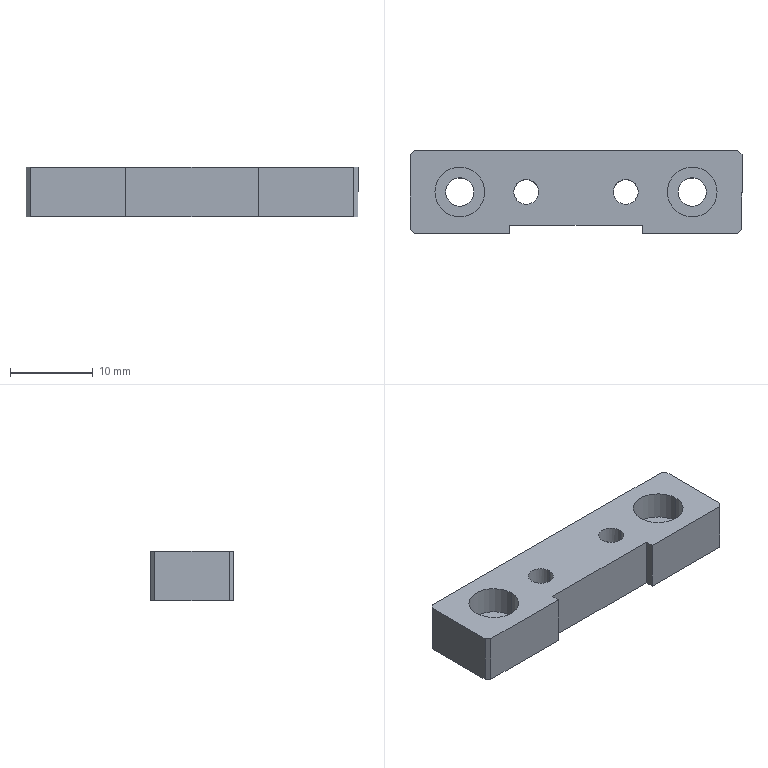Part | SolidWorks | features HoleWzd 2, Chamfer 1, Cut 1, Extrusion 1, ICE 1 | 1 solid | 32 faces | box 40 x 10 x 6 mm | volume 1941 mm3 | cylinder 16 | plane 16 | commonest cylinder face diameters 2.5 x4 3 x4 3.4 x4 6 x4
STEP:
#1=CARTESIAN_POINT('',(-6.,1.5,4.25));
#2=VERTEX_POINT('',#1);
#3=CARTESIAN_POINT('',(-6.,1.5,1.75));
#4=VERTEX_POINT('',#3);
#5=CARTESIAN_POINT('',(-6.,1.5,4.25));
#6=CARTESIAN_POINT('',(-6.088,1.5,4.25));
#7=CARTESIAN_POINT('',(-6.175,1.492,4.241));
#8=CARTESIAN_POINT('',(-6.343,1.463,4.205));
#9=CARTESIAN_POINT('',(-6.425,1.441,4.178));
#10=CARTESIAN_POINT('',(-6.653,1.36,4.079));
#11=CARTESIAN_POINT('',(-6.785,1.285,3.985));
#12=CARTESIAN_POINT('',(-7.002,1.125,3.764));
#13=CARTESIAN_POINT('',(-7.088,1.037,3.635));
#14=CARTESIAN_POINT('',(-7.181,0.9262,3.417));
#15=CARTESIAN_POINT('',(-7.206,0.8923,3.339));
#16=CARTESIAN_POINT('',(-7.241,0.8437,3.174));
#17=CARTESIAN_POINT('',(-7.25,0.8291,3.086));
#18=CARTESIAN_POINT('',(-7.25,0.8292,2.912));
#19=CARTESIAN_POINT('',(-7.24,0.844,2.824));
#20=CARTESIAN_POINT('',(-7.206,0.8927,2.66));
#21=CARTESIAN_POINT('',(-7.181,0.9265,2.582));
#22=CARTESIAN_POINT('',(-7.087,1.038,2.364));
#23=CARTESIAN_POINT('',(-7.001,1.125,2.235));
#24=CARTESIAN_POINT('',(-6.839,1.245,2.07));
#25=CARTESIAN_POINT('',(-6.779,1.284,2.019));
#26=CARTESIAN_POINT('',(-6.648,1.355,1.928));
#27=CARTESIAN_POINT('',(-6.576,1.387,1.888));
#28=CARTESIAN_POINT('',(-6.424,1.441,1.821));
#29=CARTESIAN_POINT('',(-6.342,1.463,1.795));
#30=CARTESIAN_POINT('',(-6.174,1.492,1.759));
#31=CARTESIAN_POINT('',(-6.088,1.5,1.75));
#32=CARTESIAN_POINT('',(-6.,1.5,1.75));
#33=B_SPLINE_CURVE_WITH_KNOTS('',3,(#5,#6,#7,#8,#9,#10,#11,#12,#13,#14,#15,#16,#17,#18,#19,#20,#21,#22,#23,#24,#25,#26,#27,#28,#29,#30,#31,#32),.UNSPECIFIED.,.F.,.F.,(4,2,2,2,2,2,2,2,2,2,2,2,2,4),(0.,0.0002609,0.0005218,0.001044,0.001565,0.001826,0.002087,0.002348,0.002609,0.003131,0.003391,0.003652,0.003913,0.004174),.UNSPECIFIED.);
#34=EDGE_CURVE('',#2,#4,#33,.T.);
#35=ORIENTED_EDGE('',*,*,#34,.T.);
#36=CARTESIAN_POINT('',(-6.,5.,1.75));
#37=VERTEX_POINT('',#36);
#38=CARTESIAN_POINT('',(-6.,5.,1.75));
#39=DIRECTION('',(0.,1.,0.));
#40=VECTOR('',#39,1000.);
#41=LINE('',#38,#40);
#42=EDGE_CURVE('',#4,#37,#41,.T.);
#43=ORIENTED_EDGE('',*,*,#42,.T.);
#44=CARTESIAN_POINT('',(-6.,5.,4.25));
#45=VERTEX_POINT('',#44);
#46=CARTESIAN_POINT('',(-6.,5.,3.));
#47=DIRECTION('',(0.,1.,0.));
#48=DIRECTION('',(0.,0.,1.));
#49=AXIS2_PLACEMENT_3D('',#46,#47,#48);
#50=CIRCLE('',#49,1.25);
#51=EDGE_CURVE('',#37,#45,#50,.T.);
#52=ORIENTED_EDGE('',*,*,#51,.T.);
#53=CARTESIAN_POINT('',(-6.,5.,4.25));
#54=DIRECTION('',(0.,1.,0.));
#55=VECTOR('',#54,1000.);
#56=LINE('',#53,#55);
#57=EDGE_CURVE('',#2,#45,#56,.T.);
#58=ORIENTED_EDGE('',*,*,#57,.F.);
#59=EDGE_LOOP('',(#35,#43,#52,#58));
#60=FACE_OUTER_BOUND('',#59,.T.);
#61=CARTESIAN_POINT('',(-6.,5.,3.));
#62=DIRECTION('',(0.,1.,0.));
#63=DIRECTION('',(0.,0.,1.));
#64=AXIS2_PLACEMENT_3D('',#61,#62,#63);
#65=CYLINDRICAL_SURFACE('',#64,1.25);
#66=ADVANCED_FACE('',(#60),#65,.F.);
#67=CARTESIAN_POINT('',(6.,1.5,4.25));
#68=VERTEX_POINT('',#67);
#69=CARTESIAN_POINT('',(6.,1.5,1.75));
#70=VERTEX_POINT('',#69);
#71=CARTESIAN_POINT('',(6.,1.5,4.25));
#72=CARTESIAN_POINT('',(5.912,1.5,4.25));
#73=CARTESIAN_POINT('',(5.825,1.492,4.241));
#74=CARTESIAN_POINT('',(5.657,1.463,4.205));
#75=CARTESIAN_POINT('',(5.575,1.441,4.178));
#76=CARTESIAN_POINT('',(5.347,1.36,4.079));
#77=CARTESIAN_POINT('',(5.215,1.285,3.985));
#78=CARTESIAN_POINT('',(4.998,1.125,3.764));
#79=CARTESIAN_POINT('',(4.912,1.037,3.635));
#80=CARTESIAN_POINT('',(4.819,0.9262,3.417));
#81=CARTESIAN_POINT('',(4.794,0.8923,3.339));
#82=CARTESIAN_POINT('',(4.759,0.8437,3.174));
#83=CARTESIAN_POINT('',(4.75,0.8291,3.086));
#84=CARTESIAN_POINT('',(4.75,0.8292,2.912));
#85=CARTESIAN_POINT('',(4.76,0.844,2.824));
#86=CARTESIAN_POINT('',(4.794,0.8927,2.66));
#87=CARTESIAN_POINT('',(4.819,0.9265,2.582));
#88=CARTESIAN_POINT('',(4.913,1.038,2.364));
#89=CARTESIAN_POINT('',(4.999,1.125,2.235));
#90=CARTESIAN_POINT('',(5.161,1.245,2.07));
#91=CARTESIAN_POINT('',(5.221,1.284,2.019));
#92=CARTESIAN_POINT('',(5.352,1.355,1.928));
#93=CARTESIAN_POINT('',(5.424,1.387,1.888));
#94=CARTESIAN_POINT('',(5.576,1.441,1.821));
#95=CARTESIAN_POINT('',(5.658,1.463,1.795));
#96=CARTESIAN_POINT('',(5.826,1.492,1.759));
#97=CARTESIAN_POINT('',(5.912,1.5,1.75));
#98=CARTESIAN_POINT('',(6.,1.5,1.75));
#99=B_SPLINE_CURVE_WITH_KNOTS('',3,(#71,#72,#73,#74,#75,#76,#77,#78,#79,#80,#81,#82,#83,#84,#85,#86,#87,#88,#89,#90,#91,#92,#93,#94,#95,#96,#97,#98),.UNSPECIFIED.,.F.,.F.,(4,2,2,2,2,2,2,2,2,2,2,2,2,4),(0.,0.0002609,0.0005218,0.001044,0.001565,0.001826,0.002087,0.002348,0.002609,0.003131,0.003391,0.003652,0.003913,0.004174),.UNSPECIFIED.);
#100=EDGE_CURVE('',#68,#70,#99,.T.);
#101=ORIENTED_EDGE('',*,*,#100,.T.);
#102=CARTESIAN_POINT('',(6.,5.,1.75));
#103=VERTEX_POINT('',#102);
#104=CARTESIAN_POINT('',(6.,5.,1.75));
#105=DIRECTION('',(0.,1.,0.));
#106=VECTOR('',#105,1000.);
#107=LINE('',#104,#106);
#108=EDGE_CURVE('',#70,#103,#107,.T.);
#109=ORIENTED_EDGE('',*,*,#108,.T.);
#110=CARTESIAN_POINT('',(6.,5.,4.25));
#111=VERTEX_POINT('',#110);
#112=CARTESIAN_POINT('',(6.,5.,3.));
#113=DIRECTION('',(0.,1.,0.));
#114=DIRECTION('',(0.,0.,1.));
#115=AXIS2_PLACEMENT_3D('',#112,#113,#114);
#116=CIRCLE('',#115,1.25);
#117=EDGE_CURVE('',#103,#111,#116,.T.);
#118=ORIENTED_EDGE('',*,*,#117,.T.);
#119=CARTESIAN_POINT('',(6.,5.,4.25));
#120=DIRECTION('',(0.,1.,0.));
#121=VECTOR('',#120,1000.);
#122=LINE('',#119,#121);
#123=EDGE_CURVE('',#68,#111,#122,.T.);
#124=ORIENTED_EDGE('',*,*,#123,.F.);
#125=EDGE_LOOP('',(#101,#109,#118,#124));
#126=FACE_OUTER_BOUND('',#125,.T.);
#127=CARTESIAN_POINT('',(6.,5.,3.));
#128=DIRECTION('',(0.,1.,0.));
#129=DIRECTION('',(0.,0.,1.));
#130=AXIS2_PLACEMENT_3D('',#127,#128,#129);
#131=CYLINDRICAL_SURFACE('',#130,1.25);
#132=ADVANCED_FACE('',(#126),#131,.F.);
#133=CARTESIAN_POINT('',(4.5,0.,6.));
#134=VERTEX_POINT('',#133);
#135=CARTESIAN_POINT('',(7.5,0.,6.));
#136=VERTEX_POINT('',#135);
#137=CARTESIAN_POINT('',(6.,0.,6.));
#138=DIRECTION('',(0.,0.,1.));
#139=DIRECTION('',(1.,0.,0.));
#140=AXIS2_PLACEMENT_3D('',#137,#138,#139);
#141=CIRCLE('',#140,1.5);
#142=EDGE_CURVE('',#134,#136,#141,.T.);
#143=ORIENTED_EDGE('',*,*,#142,.T.);
#144=CARTESIAN_POINT('',(7.5,0.,0.));
#145=VERTEX_POINT('',#144);
#146=CARTESIAN_POINT('',(7.5,0.,6.));
#147=DIRECTION('',(0.,0.,-1.));
#148=VECTOR('',#147,1000.);
#149=LINE('',#146,#148);
#150=EDGE_CURVE('',#136,#145,#149,.T.);
#151=ORIENTED_EDGE('',*,*,#150,.T.);
#152=CARTESIAN_POINT('',(4.5,0.,0.));
#153=VERTEX_POINT('',#152);
#154=CARTESIAN_POINT('',(6.,0.,0.));
#155=DIRECTION('',(0.,0.,1.));
#156=DIRECTION('',(1.,0.,0.));
#157=AXIS2_PLACEMENT_3D('',#154,#155,#156);
#158=CIRCLE('',#157,1.5);
#159=EDGE_CURVE('',#153,#145,#158,.T.);
#160=ORIENTED_EDGE('',*,*,#159,.F.);
#161=CARTESIAN_POINT('',(4.5,0.,6.));
#162=DIRECTION('',(0.,0.,-1.));
#163=VECTOR('',#162,1000.);
#164=LINE('',#161,#163);
#165=EDGE_CURVE('',#134,#153,#164,.T.);
#166=ORIENTED_EDGE('',*,*,#165,.F.);
#167=EDGE_LOOP('',(#143,#151,#160,#166));
#168=FACE_OUTER_BOUND('',#167,.T.);
#169=CARTESIAN_POINT('',(6.,0.,6.));
#170=DIRECTION('',(0.,0.,-1.));
#171=DIRECTION('',(-1.,0.,0.));
#172=AXIS2_PLACEMENT_3D('',#169,#170,#171);
#173=CYLINDRICAL_SURFACE('',#172,1.5);
#174=ADVANCED_FACE('',(#168),#173,.F.);
#175=CARTESIAN_POINT('',(-7.5,0.,6.));
#176=VERTEX_POINT('',#175);
#177=CARTESIAN_POINT('',(-4.5,0.,6.));
#178=VERTEX_POINT('',#177);
#179=CARTESIAN_POINT('',(-6.,0.,6.));
#180=DIRECTION('',(0.,0.,1.));
#181=DIRECTION('',(1.,0.,0.));
#182=AXIS2_PLACEMENT_3D('',#179,#180,#181);
#183=CIRCLE('',#182,1.5);
#184=EDGE_CURVE('',#176,#178,#183,.T.);
#185=ORIENTED_EDGE('',*,*,#184,.T.);
#186=CARTESIAN_POINT('',(-4.5,0.,0.));
#187=VERTEX_POINT('',#186);
#188=CARTESIAN_POINT('',(-4.5,0.,6.));
#189=DIRECTION('',(0.,0.,-1.));
#190=VECTOR('',#189,1000.);
#191=LINE('',#188,#190);
#192=EDGE_CURVE('',#178,#187,#191,.T.);
#193=ORIENTED_EDGE('',*,*,#192,.T.);
#194=CARTESIAN_POINT('',(-7.5,0.,0.));
#195=VERTEX_POINT('',#194);
#196=CARTESIAN_POINT('',(-6.,0.,0.));
#197=DIRECTION('',(0.,0.,1.));
#198=DIRECTION('',(1.,0.,0.));
#199=AXIS2_PLACEMENT_3D('',#196,#197,#198);
#200=CIRCLE('',#199,1.5);
#201=EDGE_CURVE('',#195,#187,#200,.T.);
#202=ORIENTED_EDGE('',*,*,#201,.F.);
#203=CARTESIAN_POINT('',(-7.5,0.,6.));
#204=DIRECTION('',(0.,0.,-1.));
#205=VECTOR('',#204,1000.);
#206=LINE('',#203,#205);
#207=EDGE_CURVE('',#176,#195,#206,.T.);
#208=ORIENTED_EDGE('',*,*,#207,.F.);
#209=EDGE_LOOP('',(#185,#193,#202,#208));
#210=FACE_OUTER_BOUND('',#209,.T.);
#211=CARTESIAN_POINT('',(-6.,0.,6.));
#212=DIRECTION('',(0.,0.,-1.));
#213=DIRECTION('',(-1.,0.,0.));
#214=AXIS2_PLACEMENT_3D('',#211,#212,#213);
#215=CYLINDRICAL_SURFACE('',#214,1.5);
#216=ADVANCED_FACE('',(#210),#215,.F.);
#217=CARTESIAN_POINT('',(-17.,0.,2.6));
#218=VERTEX_POINT('',#217);
#219=CARTESIAN_POINT('',(-11.,0.,2.6));
#220=VERTEX_POINT('',#219);
#221=CARTESIAN_POINT('',(-14.,0.,2.6));
#222=DIRECTION('',(0.,0.,1.));
#223=DIRECTION('',(1.,0.,0.));
#224=AXIS2_PLACEMENT_3D('',#221,#222,#223);
#225=CIRCLE('',#224,3.);
#226=EDGE_CURVE('',#218,#220,#225,.T.);
#227=ORIENTED_EDGE('',*,*,#226,.F.);
#228=CARTESIAN_POINT('',(-17.,0.,6.));
#229=VERTEX_POINT('',#228);
#230=CARTESIAN_POINT('',(-17.,0.,6.));
#231=DIRECTION('',(0.,0.,1.));
#232=VECTOR('',#231,1000.);
#233=LINE('',#230,#232);
#234=EDGE_CURVE('',#218,#229,#233,.T.);
#235=ORIENTED_EDGE('',*,*,#234,.T.);
#236=CARTESIAN_POINT('',(-11.,0.,6.));
#237=VERTEX_POINT('',#236);
#238=CARTESIAN_POINT('',(-14.,0.,6.));
#239=DIRECTION('',(0.,0.,1.));
#240=DIRECTION('',(1.,0.,0.));
#241=AXIS2_PLACEMENT_3D('',#238,#239,#240);
#242=CIRCLE('',#241,3.);
#243=EDGE_CURVE('',#229,#237,#242,.T.);
#244=ORIENTED_EDGE('',*,*,#243,.T.);
#245=CARTESIAN_POINT('',(-11.,0.,6.));
#246=DIRECTION('',(0.,0.,1.));
#247=VECTOR('',#246,1000.);
#248=LINE('',#245,#247);
#249=EDGE_CURVE('',#220,#237,#248,.T.);
#250=ORIENTED_EDGE('',*,*,#249,.F.);
#251=EDGE_LOOP('',(#227,#235,#244,#250));
#252=FACE_OUTER_BOUND('',#251,.T.);
#253=CARTESIAN_POINT('',(-14.,0.,6.));
#254=DIRECTION('',(0.,0.,1.));
#255=DIRECTION('',(1.,0.,0.));
#256=AXIS2_PLACEMENT_3D('',#253,#254,#255);
#257=CYLINDRICAL_SURFACE('',#256,3.);
#258=ADVANCED_FACE('',(#252),#257,.F.);
#259=CARTESIAN_POINT('',(-15.7,0.,0.));
#260=VERTEX_POINT('',#259);
#261=CARTESIAN_POINT('',(-12.3,0.,0.));
#262=VERTEX_POINT('',#261);
#263=CARTESIAN_POINT('',(-14.,0.,0.));
#264=DIRECTION('',(0.,0.,1.));
#265=DIRECTION('',(1.,0.,0.));
#266=AXIS2_PLACEMENT_3D('',#263,#264,#265);
#267=CIRCLE('',#266,1.7);
#268=EDGE_CURVE('',#260,#262,#267,.T.);
#269=ORIENTED_EDGE('',*,*,#268,.F.);
#270=CARTESIAN_POINT('',(-15.7,0.,2.6));
#271=VERTEX_POINT('',#270);
#272=CARTESIAN_POINT('',(-15.7,0.,6.));
#273=DIRECTION('',(0.,0.,1.));
#274=VECTOR('',#273,1000.);
#275=LINE('',#272,#274);
#276=EDGE_CURVE('',#260,#271,#275,.T.);
#277=ORIENTED_EDGE('',*,*,#276,.T.);
#278=CARTESIAN_POINT('',(-12.3,0.,2.6));
#279=VERTEX_POINT('',#278);
#280=CARTESIAN_POINT('',(-14.,0.,2.6));
#281=DIRECTION('',(0.,0.,1.));
#282=DIRECTION('',(1.,0.,0.));
#283=AXIS2_PLACEMENT_3D('',#280,#281,#282);
#284=CIRCLE('',#283,1.7);
#285=EDGE_CURVE('',#271,#279,#284,.T.);
#286=ORIENTED_EDGE('',*,*,#285,.T.);
#287=CARTESIAN_POINT('',(-12.3,0.,6.));
#288=DIRECTION('',(0.,0.,1.));
#289=VECTOR('',#288,1000.);
#290=LINE('',#287,#289);
#291=EDGE_CURVE('',#262,#279,#290,.T.);
#292=ORIENTED_EDGE('',*,*,#291,.F.);
#293=EDGE_LOOP('',(#269,#277,#286,#292));
#294=FACE_OUTER_BOUND('',#293,.T.);
#295=CARTESIAN_POINT('',(-14.,0.,6.));
#296=DIRECTION('',(0.,0.,1.));
#297=DIRECTION('',(1.,0.,0.));
#298=AXIS2_PLACEMENT_3D('',#295,#296,#297);
#299=CYLINDRICAL_SURFACE('',#298,1.7);
#300=ADVANCED_FACE('',(#294),#299,.F.);
#301=CARTESIAN_POINT('',(11.,0.,2.6));
#302=VERTEX_POINT('',#301);
#303=CARTESIAN_POINT('',(17.,0.,2.6));
#304=VERTEX_POINT('',#303);
#305=CARTESIAN_POINT('',(14.,0.,2.6));
#306=DIRECTION('',(0.,0.,1.));
#307=DIRECTION('',(1.,0.,0.));
#308=AXIS2_PLACEMENT_3D('',#305,#306,#307);
#309=CIRCLE('',#308,3.);
#310=EDGE_CURVE('',#302,#304,#309,.T.);
#311=ORIENTED_EDGE('',*,*,#310,.F.);
#312=CARTESIAN_POINT('',(11.,0.,6.));
#313=VERTEX_POINT('',#312);
#314=CARTESIAN_POINT('',(11.,0.,6.));
#315=DIRECTION('',(0.,0.,1.));
#316=VECTOR('',#315,1000.);
#317=LINE('',#314,#316);
#318=EDGE_CURVE('',#302,#313,#317,.T.);
#319=ORIENTED_EDGE('',*,*,#318,.T.);
#320=CARTESIAN_POINT('',(17.,0.,6.));
#321=VERTEX_POINT('',#320);
#322=CARTESIAN_POINT('',(14.,0.,6.));
#323=DIRECTION('',(0.,0.,1.));
#324=DIRECTION('',(1.,0.,0.));
#325=AXIS2_PLACEMENT_3D('',#322,#323,#324);
#326=CIRCLE('',#325,3.);
#327=EDGE_CURVE('',#313,#321,#326,.T.);
#328=ORIENTED_EDGE('',*,*,#327,.T.);
#329=CARTESIAN_POINT('',(17.,0.,6.));
#330=DIRECTION('',(0.,0.,1.));
#331=VECTOR('',#330,1000.);
#332=LINE('',#329,#331);
#333=EDGE_CURVE('',#304,#321,#332,.T.);
#334=ORIENTED_EDGE('',*,*,#333,.F.);
#335=EDGE_LOOP('',(#311,#319,#328,#334));
#336=FACE_OUTER_BOUND('',#335,.T.);
#337=CARTESIAN_POINT('',(14.,0.,6.));
#338=DIRECTION('',(0.,0.,1.));
#339=DIRECTION('',(1.,0.,0.));
#340=AXIS2_PLACEMENT_3D('',#337,#338,#339);
#341=CYLINDRICAL_SURFACE('',#340,3.);
#342=ADVANCED_FACE('',(#336),#341,.F.);
#343=CARTESIAN_POINT('',(12.3,0.,0.));
#344=VERTEX_POINT('',#343);
#345=CARTESIAN_POINT('',(15.7,0.,0.));
#346=VERTEX_POINT('',#345);
#347=CARTESIAN_POINT('',(14.,0.,0.));
#348=DIRECTION('',(0.,0.,1.));
#349=DIRECTION('',(1.,0.,0.));
#350=AXIS2_PLACEMENT_3D('',#347,#348,#349);
#351=CIRCLE('',#350,1.7);
#352=EDGE_CURVE('',#344,#346,#351,.T.);
#353=ORIENTED_EDGE('',*,*,#352,.F.);
#354=CARTESIAN_POINT('',(12.3,0.,2.6));
#355=VERTEX_POINT('',#354);
#356=CARTESIAN_POINT('',(12.3,0.,6.));
#357=DIRECTION('',(0.,0.,1.));
#358=VECTOR('',#357,1000.);
#359=LINE('',#356,#358);
#360=EDGE_CURVE('',#344,#355,#359,.T.);
#361=ORIENTED_EDGE('',*,*,#360,.T.);
#362=CARTESIAN_POINT('',(15.7,0.,2.6));
#363=VERTEX_POINT('',#362);
#364=CARTESIAN_POINT('',(14.,0.,2.6));
#365=DIRECTION('',(0.,0.,1.));
#366=DIRECTION('',(1.,0.,0.));
#367=AXIS2_PLACEMENT_3D('',#364,#365,#366);
#368=CIRCLE('',#367,1.7);
#369=EDGE_CURVE('',#355,#363,#368,.T.);
#370=ORIENTED_EDGE('',*,*,#369,.T.);
#371=CARTESIAN_POINT('',(15.7,0.,6.));
#372=DIRECTION('',(0.,0.,1.));
#373=VECTOR('',#372,1000.);
#374=LINE('',#371,#373);
#375=EDGE_CURVE('',#346,#363,#374,.T.);
#376=ORIENTED_EDGE('',*,*,#375,.F.);
#377=EDGE_LOOP('',(#353,#361,#370,#376));
#378=FACE_OUTER_BOUND('',#377,.T.);
#379=CARTESIAN_POINT('',(14.,0.,6.));
#380=DIRECTION('',(0.,0.,1.));
#381=DIRECTION('',(1.,0.,0.));
#382=AXIS2_PLACEMENT_3D('',#379,#380,#381);
#383=CYLINDRICAL_SURFACE('',#382,1.7);
#384=ADVANCED_FACE('',(#378),#383,.F.);
#385=ORIENTED_EDGE('',*,*,#184,.F.);
#386=CARTESIAN_POINT('',(-6.,0.,6.));
#387=DIRECTION('',(0.,0.,1.));
#388=DIRECTION('',(1.,0.,0.));
#389=AXIS2_PLACEMENT_3D('',#386,#387,#388);
#390=CIRCLE('',#389,1.5);
#391=EDGE_CURVE('',#178,#176,#390,.T.);
#392=ORIENTED_EDGE('',*,*,#391,.F.);
#393=EDGE_LOOP('',(#385,#392));
#394=FACE_BOUND('',#393,.T.);
#395=CARTESIAN_POINT('',(14.,0.,6.));
#396=DIRECTION('',(0.,0.,1.));
#397=DIRECTION('',(1.,0.,0.));
#398=AXIS2_PLACEMENT_3D('',#395,#396,#397);
#399=CIRCLE('',#398,3.);
#400=EDGE_CURVE('',#321,#313,#399,.T.);
#401=ORIENTED_EDGE('',*,*,#400,.F.);
#402=ORIENTED_EDGE('',*,*,#327,.F.);
#403=EDGE_LOOP('',(#401,#402));
#404=FACE_BOUND('',#403,.T.);
#405=CARTESIAN_POINT('',(-14.,0.,6.));
#406=DIRECTION('',(0.,0.,1.));
#407=DIRECTION('',(1.,0.,0.));
#408=AXIS2_PLACEMENT_3D('',#405,#406,#407);
#409=CIRCLE('',#408,3.);
#410=EDGE_CURVE('',#237,#229,#409,.T.);
#411=ORIENTED_EDGE('',*,*,#410,.F.);
#412=ORIENTED_EDGE('',*,*,#243,.F.);
#413=EDGE_LOOP('',(#411,#412));
#414=FACE_BOUND('',#413,.T.);
#415=CARTESIAN_POINT('',(-19.5,-5.,6.));
#416=VERTEX_POINT('',#415);
#417=CARTESIAN_POINT('',(-8.,-5.,6.));
#418=VERTEX_POINT('',#417);
#419=CARTESIAN_POINT('',(20.,-5.,6.));
#420=DIRECTION('',(1.,0.,0.));
#421=VECTOR('',#420,1000.);
#422=LINE('',#419,#421);
#423=EDGE_CURVE('',#416,#418,#422,.T.);
#424=ORIENTED_EDGE('',*,*,#423,.T.);
#425=CARTESIAN_POINT('',(-8.,-4.,6.));
#426=VERTEX_POINT('',#425);
#427=CARTESIAN_POINT('',(-8.,-4.,6.));
#428=DIRECTION('',(0.,-1.,0.));
#429=VECTOR('',#428,1000.);
#430=LINE('',#427,#429);
#431=EDGE_CURVE('',#426,#418,#430,.T.);
#432=ORIENTED_EDGE('',*,*,#431,.F.);
#433=CARTESIAN_POINT('',(8.,-4.,6.));
#434=VERTEX_POINT('',#433);
#435=CARTESIAN_POINT('',(8.,-4.,6.));
#436=DIRECTION('',(1.,0.,0.));
#437=VECTOR('',#436,1000.);
#438=LINE('',#435,#437);
#439=EDGE_CURVE('',#426,#434,#438,.T.);
#440=ORIENTED_EDGE('',*,*,#439,.T.);
#441=CARTESIAN_POINT('',(8.,-5.,6.));
#442=VERTEX_POINT('',#441);
#443=CARTESIAN_POINT('',(8.,-4.,6.));
#444=DIRECTION('',(0.,-1.,0.));
#445=VECTOR('',#444,1000.);
#446=LINE('',#443,#445);
#447=EDGE_CURVE('',#434,#442,#446,.T.);
#448=ORIENTED_EDGE('',*,*,#447,.T.);
#449=CARTESIAN_POINT('',(19.5,-5.,6.));
#450=VERTEX_POINT('',#449);
#451=CARTESIAN_POINT('',(20.,-5.,6.));
#452=DIRECTION('',(1.,0.,0.));
#453=VECTOR('',#452,1000.);
#454=LINE('',#451,#453);
#455=EDGE_CURVE('',#442,#450,#454,.T.);
#456=ORIENTED_EDGE('',*,*,#455,.T.);
#457=CARTESIAN_POINT('',(20.,-4.5,6.));
#458=VERTEX_POINT('',#457);
#459=CARTESIAN_POINT('',(4.75,-19.75,6.));
#460=DIRECTION('',(0.7071,0.7071,0.));
#461=VECTOR('',#460,1000.);
#462=LINE('',#459,#461);
#463=EDGE_CURVE('',#450,#458,#462,.T.);
#464=ORIENTED_EDGE('',*,*,#463,.T.);
#465=CARTESIAN_POINT('',(20.,4.5,6.));
#466=VERTEX_POINT('',#465);
#467=CARTESIAN_POINT('',(20.,-5.,6.));
#468=DIRECTION('',(0.,1.,0.));
#469=VECTOR('',#468,1000.);
#470=LINE('',#467,#469);
#471=EDGE_CURVE('',#458,#466,#470,.T.);
#472=ORIENTED_EDGE('',*,*,#471,.T.);
#473=CARTESIAN_POINT('',(19.5,5.,6.));
#474=VERTEX_POINT('',#473);
#475=CARTESIAN_POINT('',(-0.25,24.75,6.));
#476=DIRECTION('',(-0.7071,0.7071,0.));
#477=VECTOR('',#476,1000.);
#478=LINE('',#475,#477);
#479=EDGE_CURVE('',#466,#474,#478,.T.);
#480=ORIENTED_EDGE('',*,*,#479,.T.);
#481=CARTESIAN_POINT('',(-19.5,5.,6.));
#482=VERTEX_POINT('',#481);
#483=CARTESIAN_POINT('',(20.,5.,6.));
#484=DIRECTION('',(-1.,0.,0.));
#485=VECTOR('',#484,1000.);
#486=LINE('',#483,#485);
#487=EDGE_CURVE('',#474,#482,#486,.T.);
#488=ORIENTED_EDGE('',*,*,#487,.T.);
#489=CARTESIAN_POINT('',(-20.,4.5,6.));
#490=VERTEX_POINT('',#489);
#491=CARTESIAN_POINT('',(-19.75,4.75,6.));
#492=DIRECTION('',(-0.7071,-0.7071,0.));
#493=VECTOR('',#492,1000.);
#494=LINE('',#491,#493);
#495=EDGE_CURVE('',#482,#490,#494,.T.);
#496=ORIENTED_EDGE('',*,*,#495,.T.);
#497=CARTESIAN_POINT('',(-20.,-4.5,6.));
#498=VERTEX_POINT('',#497);
#499=CARTESIAN_POINT('',(-20.,-5.,6.));
#500=DIRECTION('',(0.,-1.,0.));
#501=VECTOR('',#500,1000.);
#502=LINE('',#499,#501);
#503=EDGE_CURVE('',#490,#498,#502,.T.);
#504=ORIENTED_EDGE('',*,*,#503,.T.);
#505=CARTESIAN_POINT('',(-24.75,0.25,6.));
#506=DIRECTION('',(0.7071,-0.7071,0.));
#507=VECTOR('',#506,1000.);
#508=LINE('',#505,#507);
#509=EDGE_CURVE('',#498,#416,#508,.T.);
#510=ORIENTED_EDGE('',*,*,#509,.T.);
#511=EDGE_LOOP('',(#424,#432,#440,#448,#456,#464,#472,#480,#488,#496,#504,#510));
#512=FACE_OUTER_BOUND('',#511,.T.);
#513=ORIENTED_EDGE('',*,*,#142,.F.);
#514=CARTESIAN_POINT('',(6.,0.,6.));
#515=DIRECTION('',(0.,0.,1.));
#516=DIRECTION('',(1.,0.,0.));
#517=AXIS2_PLACEMENT_3D('',#514,#515,#516);
#518=CIRCLE('',#517,1.5);
#519=EDGE_CURVE('',#136,#134,#518,.T.);
#520=ORIENTED_EDGE('',*,*,#519,.F.);
#521=EDGE_LOOP('',(#513,#520));
#522=FACE_BOUND('',#521,.T.);
#523=CARTESIAN_POINT('',(-20.,5.,6.));
#524=DIRECTION('',(0.,0.,1.));
#525=DIRECTION('',(1.,0.,0.));
#526=AXIS2_PLACEMENT_3D('',#523,#524,#525);
#527=PLANE('',#526);
#528=ADVANCED_FACE('',(#394,#404,#414,#512,#522),#527,.T.);
#529=ORIENTED_EDGE('',*,*,#201,.T.);
#530=CARTESIAN_POINT('',(-6.,0.,0.));
#531=DIRECTION('',(0.,0.,1.));
#532=DIRECTION('',(1.,0.,0.));
#533=AXIS2_PLACEMENT_3D('',#530,#531,#532);
#534=CIRCLE('',#533,1.5);
#535=EDGE_CURVE('',#187,#195,#534,.T.);
#536=ORIENTED_EDGE('',*,*,#535,.T.);
#537=EDGE_LOOP('',(#529,#536));
#538=FACE_BOUND('',#537,.T.);
#539=CARTESIAN_POINT('',(14.,0.,0.));
#540=DIRECTION('',(0.,0.,1.));
#541=DIRECTION('',(1.,0.,0.));
#542=AXIS2_PLACEMENT_3D('',#539,#540,#541);
#543=CIRCLE('',#542,1.7);
#544=EDGE_CURVE('',#346,#344,#543,.T.);
#545=ORIENTED_EDGE('',*,*,#544,.T.);
#546=ORIENTED_EDGE('',*,*,#352,.T.);
#547=EDGE_LOOP('',(#545,#546));
#548=FACE_BOUND('',#547,.T.);
#549=CARTESIAN_POINT('',(-14.,0.,0.));
#550=DIRECTION('',(0.,0.,1.));
#551=DIRECTION('',(1.,0.,0.));
#552=AXIS2_PLACEMENT_3D('',#549,#550,#551);
#553=CIRCLE('',#552,1.7);
#554=EDGE_CURVE('',#262,#260,#553,.T.);
#555=ORIENTED_EDGE('',*,*,#554,.T.);
#556=ORIENTED_EDGE('',*,*,#268,.T.);
#557=EDGE_LOOP('',(#555,#556));
#558=FACE_BOUND('',#557,.T.);
#559=CARTESIAN_POINT('',(-8.,-4.,0.));
#560=VERTEX_POINT('',#559);
#561=CARTESIAN_POINT('',(-8.,-5.,0.));
#562=VERTEX_POINT('',#561);
#563=CARTESIAN_POINT('',(-8.,-4.,0.));
#564=DIRECTION('',(0.,-1.,0.));
#565=VECTOR('',#564,1000.);
#566=LINE('',#563,#565);
#567=EDGE_CURVE('',#560,#562,#566,.T.);
#568=ORIENTED_EDGE('',*,*,#567,.T.);
#569=CARTESIAN_POINT('',(-19.5,-5.,0.));
#570=VERTEX_POINT('',#569);
#571=CARTESIAN_POINT('',(20.,-5.,0.));
#572=DIRECTION('',(1.,0.,0.));
#573=VECTOR('',#572,1000.);
#574=LINE('',#571,#573);
#575=EDGE_CURVE('',#570,#562,#574,.T.);
#576=ORIENTED_EDGE('',*,*,#575,.F.);
#577=CARTESIAN_POINT('',(-20.,-4.5,0.));
#578=VERTEX_POINT('',#577);
#579=CARTESIAN_POINT('',(-19.5,-5.,0.));
#580=DIRECTION('',(-0.7071,0.7071,0.));
#581=VECTOR('',#580,1000.);
#582=LINE('',#579,#581);
#583=EDGE_CURVE('',#570,#578,#582,.T.);
#584=ORIENTED_EDGE('',*,*,#583,.T.);
#585=CARTESIAN_POINT('',(-20.,4.5,0.));
#586=VERTEX_POINT('',#585);
#587=CARTESIAN_POINT('',(-20.,-5.,0.));
#588=DIRECTION('',(0.,-1.,0.));
#589=VECTOR('',#588,1000.);
#590=LINE('',#587,#589);
#591=EDGE_CURVE('',#586,#578,#590,.T.);
#592=ORIENTED_EDGE('',*,*,#591,.F.);
#593=CARTESIAN_POINT('',(-19.5,5.,0.));
#594=VERTEX_POINT('',#593);
#595=CARTESIAN_POINT('',(-20.,4.5,0.));
#596=DIRECTION('',(0.7071,0.7071,0.));
#597=VECTOR('',#596,1000.);
#598=LINE('',#595,#597);
#599=EDGE_CURVE('',#586,#594,#598,.T.);
#600=ORIENTED_EDGE('',*,*,#599,.T.);
#601=CARTESIAN_POINT('',(19.5,5.,0.));
#602=VERTEX_POINT('',#601);
#603=CARTESIAN_POINT('',(20.,5.,0.));
#604=DIRECTION('',(-1.,0.,0.));
#605=VECTOR('',#604,1000.);
#606=LINE('',#603,#605);
#607=EDGE_CURVE('',#602,#594,#606,.T.);
#608=ORIENTED_EDGE('',*,*,#607,.F.);
#609=CARTESIAN_POINT('',(20.,4.5,0.));
#610=VERTEX_POINT('',#609);
#611=CARTESIAN_POINT('',(19.5,5.,0.));
#612=DIRECTION('',(0.7071,-0.7071,0.));
#613=VECTOR('',#612,1000.);
#614=LINE('',#611,#613);
#615=EDGE_CURVE('',#602,#610,#614,.T.);
#616=ORIENTED_EDGE('',*,*,#615,.T.);
#617=CARTESIAN_POINT('',(20.,-4.5,0.));
#618=VERTEX_POINT('',#617);
#619=CARTESIAN_POINT('',(20.,-5.,0.));
#620=DIRECTION('',(0.,1.,0.));
#621=VECTOR('',#620,1000.);
#622=LINE('',#619,#621);
#623=EDGE_CURVE('',#618,#610,#622,.T.);
#624=ORIENTED_EDGE('',*,*,#623,.F.);
#625=CARTESIAN_POINT('',(19.5,-5.,0.));
#626=VERTEX_POINT('',#625);
#627=CARTESIAN_POINT('',(20.,-4.5,0.));
#628=DIRECTION('',(-0.7071,-0.7071,0.));
#629=VECTOR('',#628,1000.);
#630=LINE('',#627,#629);
#631=EDGE_CURVE('',#618,#626,#630,.T.);
#632=ORIENTED_EDGE('',*,*,#631,.T.);
#633=CARTESIAN_POINT('',(8.,-5.,0.));
#634=VERTEX_POINT('',#633);
#635=CARTESIAN_POINT('',(20.,-5.,0.));
#636=DIRECTION('',(1.,0.,0.));
#637=VECTOR('',#636,1000.);
#638=LINE('',#635,#637);
#639=EDGE_CURVE('',#634,#626,#638,.T.);
#640=ORIENTED_EDGE('',*,*,#639,.F.);
#641=CARTESIAN_POINT('',(8.,-4.,0.));
#642=VERTEX_POINT('',#641);
#643=CARTESIAN_POINT('',(8.,-4.,0.));
#644=DIRECTION('',(0.,-1.,0.));
#645=VECTOR('',#644,1000.);
#646=LINE('',#643,#645);
#647=EDGE_CURVE('',#642,#634,#646,.T.);
#648=ORIENTED_EDGE('',*,*,#647,.F.);
#649=CARTESIAN_POINT('',(8.,-4.,0.));
#650=DIRECTION('',(-1.,0.,0.));
#651=VECTOR('',#650,1000.);
#652=LINE('',#649,#651);
#653=EDGE_CURVE('',#642,#560,#652,.T.);
#654=ORIENTED_EDGE('',*,*,#653,.T.);
#655=EDGE_LOOP('',(#568,#576,#584,#592,#600,#608,#616,#624,#632,#640,#648,#654));
#656=FACE_OUTER_BOUND('',#655,.T.);
#657=ORIENTED_EDGE('',*,*,#159,.T.);
#658=CARTESIAN_POINT('',(6.,0.,0.));
#659=DIRECTION('',(0.,0.,1.));
#660=DIRECTION('',(1.,0.,0.));
#661=AXIS2_PLACEMENT_3D('',#658,#659,#660);
#662=CIRCLE('',#661,1.5);
#663=EDGE_CURVE('',#145,#153,#662,.T.);
#664=ORIENTED_EDGE('',*,*,#663,.T.);
#665=EDGE_LOOP('',(#657,#664));
#666=FACE_BOUND('',#665,.T.);
#667=CARTESIAN_POINT('',(-20.,5.,0.));
#668=DIRECTION('',(0.,0.,1.));
#669=DIRECTION('',(1.,0.,0.));
#670=AXIS2_PLACEMENT_3D('',#667,#668,#669);
#671=PLANE('',#670);
#672=ADVANCED_FACE('',(#538,#548,#558,#656,#666),#671,.F.);
#673=CARTESIAN_POINT('',(-8.,-5.,6.));
#674=DIRECTION('',(0.,0.,1.));
#675=VECTOR('',#674,1000.);
#676=LINE('',#673,#675);
#677=EDGE_CURVE('',#562,#418,#676,.T.);
#678=ORIENTED_EDGE('',*,*,#677,.T.);
#679=ORIENTED_EDGE('',*,*,#423,.F.);
#680=CARTESIAN_POINT('',(-19.5,-5.,6.));
#681=DIRECTION('',(0.,0.,-1.));
#682=VECTOR('',#681,1000.);
#683=LINE('',#680,#682);
#684=EDGE_CURVE('',#416,#570,#683,.T.);
#685=ORIENTED_EDGE('',*,*,#684,.T.);
#686=ORIENTED_EDGE('',*,*,#575,.T.);
#687=EDGE_LOOP('',(#678,#679,#685,#686));
#688=FACE_OUTER_BOUND('',#687,.T.);
#689=CARTESIAN_POINT('',(20.,-5.,6.));
#690=DIRECTION('',(0.,1.,0.));
#691=DIRECTION('',(-1.,0.,0.));
#692=AXIS2_PLACEMENT_3D('',#689,#690,#691);
#693=PLANE('',#692);
#694=ADVANCED_FACE('',(#688),#693,.F.);
#695=CARTESIAN_POINT('',(8.,-5.,6.));
#696=DIRECTION('',(0.,0.,-1.));
#697=VECTOR('',#696,1000.);
#698=LINE('',#695,#697);
#699=EDGE_CURVE('',#442,#634,#698,.T.);
#700=ORIENTED_EDGE('',*,*,#699,.T.);
#701=ORIENTED_EDGE('',*,*,#639,.T.);
#702=CARTESIAN_POINT('',(19.5,-5.,6.));
#703=DIRECTION('',(0.,0.,1.));
#704=VECTOR('',#703,1000.);
#705=LINE('',#702,#704);
#706=EDGE_CURVE('',#626,#450,#705,.T.);
#707=ORIENTED_EDGE('',*,*,#706,.T.);
#708=ORIENTED_EDGE('',*,*,#455,.F.);
#709=EDGE_LOOP('',(#700,#701,#707,#708));
#710=FACE_OUTER_BOUND('',#709,.T.);
#711=CARTESIAN_POINT('',(20.,-5.,6.));
#712=DIRECTION('',(0.,1.,0.));
#713=DIRECTION('',(-1.,0.,0.));
#714=AXIS2_PLACEMENT_3D('',#711,#712,#713);
#715=PLANE('',#714);
#716=ADVANCED_FACE('',(#710),#715,.F.);
#717=ORIENTED_EDGE('',*,*,#503,.F.);
#718=CARTESIAN_POINT('',(-20.,4.5,6.));
#719=DIRECTION('',(0.,0.,-1.));
#720=VECTOR('',#719,1000.);
#721=LINE('',#718,#720);
#722=EDGE_CURVE('',#490,#586,#721,.T.);
#723=ORIENTED_EDGE('',*,*,#722,.T.);
#724=ORIENTED_EDGE('',*,*,#591,.T.);
#725=CARTESIAN_POINT('',(-20.,-4.5,6.));
#726=DIRECTION('',(0.,0.,1.));
#727=VECTOR('',#726,1000.);
#728=LINE('',#725,#727);
#729=EDGE_CURVE('',#578,#498,#728,.T.);
#730=ORIENTED_EDGE('',*,*,#729,.T.);
#731=EDGE_LOOP('',(#717,#723,#724,#730));
#732=FACE_OUTER_BOUND('',#731,.T.);
#733=CARTESIAN_POINT('',(-20.,-5.,6.));
#734=DIRECTION('',(1.,0.,0.));
#735=DIRECTION('',(0.,0.,-1.));
#736=AXIS2_PLACEMENT_3D('',#733,#734,#735);
#737=PLANE('',#736);
#738=ADVANCED_FACE('',(#732),#737,.F.);
#739=ORIENTED_EDGE('',*,*,#471,.F.);
#740=CARTESIAN_POINT('',(20.,-4.5,6.));
#741=DIRECTION('',(0.,0.,-1.));
#742=VECTOR('',#741,1000.);
#743=LINE('',#740,#742);
#744=EDGE_CURVE('',#458,#618,#743,.T.);
#745=ORIENTED_EDGE('',*,*,#744,.T.);
#746=ORIENTED_EDGE('',*,*,#623,.T.);
#747=CARTESIAN_POINT('',(20.,4.5,6.));
#748=DIRECTION('',(0.,0.,1.));
#749=VECTOR('',#748,1000.);
#750=LINE('',#747,#749);
#751=EDGE_CURVE('',#610,#466,#750,.T.);
#752=ORIENTED_EDGE('',*,*,#751,.T.);
#753=EDGE_LOOP('',(#739,#745,#746,#752));
#754=FACE_OUTER_BOUND('',#753,.T.);
#755=CARTESIAN_POINT('',(20.,-5.,6.));
#756=DIRECTION('',(-1.,0.,0.));
#757=DIRECTION('',(0.,0.,1.));
#758=AXIS2_PLACEMENT_3D('',#755,#756,#757);
#759=PLANE('',#758);
#760=ADVANCED_FACE('',(#754),#759,.F.);
#761=CARTESIAN_POINT('',(-6.,5.,3.));
#762=DIRECTION('',(0.,1.,0.));
#763=DIRECTION('',(0.,0.,1.));
#764=AXIS2_PLACEMENT_3D('',#761,#762,#763);
#765=CIRCLE('',#764,1.25);
#766=EDGE_CURVE('',#45,#37,#765,.T.);
#767=ORIENTED_EDGE('',*,*,#766,.F.);
#768=ORIENTED_EDGE('',*,*,#51,.F.);
#769=EDGE_LOOP('',(#767,#768));
#770=FACE_BOUND('',#769,.T.);
#771=CARTESIAN_POINT('',(6.,5.,3.));
#772=DIRECTION('',(0.,1.,0.));
#773=DIRECTION('',(0.,0.,1.));
#774=AXIS2_PLACEMENT_3D('',#771,#772,#773);
#775=CIRCLE('',#774,1.25);
#776=EDGE_CURVE('',#111,#103,#775,.T.);
#777=ORIENTED_EDGE('',*,*,#776,.F.);
#778=ORIENTED_EDGE('',*,*,#117,.F.);
#779=EDGE_LOOP('',(#777,#778));
#780=FACE_BOUND('',#779,.T.);
#781=ORIENTED_EDGE('',*,*,#487,.F.);
#782=CARTESIAN_POINT('',(19.5,5.,6.));
#783=DIRECTION('',(0.,0.,-1.));
#784=VECTOR('',#783,1000.);
#785=LINE('',#782,#784);
#786=EDGE_CURVE('',#474,#602,#785,.T.);
#787=ORIENTED_EDGE('',*,*,#786,.T.);
#788=ORIENTED_EDGE('',*,*,#607,.T.);
#789=CARTESIAN_POINT('',(-19.5,5.,6.));
#790=DIRECTION('',(0.,0.,1.));
#791=VECTOR('',#790,1000.);
#792=LINE('',#789,#791);
#793=EDGE_CURVE('',#594,#482,#792,.T.);
#794=ORIENTED_EDGE('',*,*,#793,.T.);
#795=EDGE_LOOP('',(#781,#787,#788,#794));
#796=FACE_OUTER_BOUND('',#795,.T.);
#797=CARTESIAN_POINT('',(20.,5.,6.));
#798=DIRECTION('',(0.,-1.,0.));
#799=DIRECTION('',(1.,0.,0.));
#800=AXIS2_PLACEMENT_3D('',#797,#798,#799);
#801=PLANE('',#800);
#802=ADVANCED_FACE('',(#770,#780,#796),#801,.F.);
#803=ORIENTED_EDGE('',*,*,#463,.F.);
#804=ORIENTED_EDGE('',*,*,#706,.F.);
#805=ORIENTED_EDGE('',*,*,#631,.F.);
#806=ORIENTED_EDGE('',*,*,#744,.F.);
#807=EDGE_LOOP('',(#803,#804,#805,#806));
#808=FACE_OUTER_BOUND('',#807,.T.);
#809=CARTESIAN_POINT('',(20.,-4.5,6.));
#810=DIRECTION('',(-0.7071,0.7071,0.));
#811=DIRECTION('',(-0.7071,-0.7071,0.));
#812=AXIS2_PLACEMENT_3D('',#809,#810,#811);
#813=PLANE('',#812);
#814=ADVANCED_FACE('',(#808),#813,.F.);
#815=ORIENTED_EDGE('',*,*,#479,.F.);
#816=ORIENTED_EDGE('',*,*,#751,.F.);
#817=ORIENTED_EDGE('',*,*,#615,.F.);
#818=ORIENTED_EDGE('',*,*,#786,.F.);
#819=EDGE_LOOP('',(#815,#816,#817,#818));
#820=FACE_OUTER_BOUND('',#819,.T.);
#821=CARTESIAN_POINT('',(19.5,5.,6.));
#822=DIRECTION('',(-0.7071,-0.7071,0.));
#823=DIRECTION('',(0.7071,-0.7071,0.));
#824=AXIS2_PLACEMENT_3D('',#821,#822,#823);
#825=PLANE('',#824);
#826=ADVANCED_FACE('',(#820),#825,.F.);
#827=ORIENTED_EDGE('',*,*,#495,.F.);
#828=ORIENTED_EDGE('',*,*,#793,.F.);
#829=ORIENTED_EDGE('',*,*,#599,.F.);
#830=ORIENTED_EDGE('',*,*,#722,.F.);
#831=EDGE_LOOP('',(#827,#828,#829,#830));
#832=FACE_OUTER_BOUND('',#831,.T.);
#833=CARTESIAN_POINT('',(-20.,4.5,6.));
#834=DIRECTION('',(0.7071,-0.7071,0.));
#835=DIRECTION('',(0.7071,0.7071,0.));
#836=AXIS2_PLACEMENT_3D('',#833,#834,#835);
#837=PLANE('',#836);
#838=ADVANCED_FACE('',(#832),#837,.F.);
#839=ORIENTED_EDGE('',*,*,#509,.F.);
#840=ORIENTED_EDGE('',*,*,#729,.F.);
#841=ORIENTED_EDGE('',*,*,#583,.F.);
#842=ORIENTED_EDGE('',*,*,#684,.F.);
#843=EDGE_LOOP('',(#839,#840,#841,#842));
#844=FACE_OUTER_BOUND('',#843,.T.);
#845=CARTESIAN_POINT('',(-19.5,-5.,6.));
#846=DIRECTION('',(0.7071,0.7071,0.));
#847=DIRECTION('',(-0.7071,0.7071,0.));
#848=AXIS2_PLACEMENT_3D('',#845,#846,#847);
#849=PLANE('',#848);
#850=ADVANCED_FACE('',(#844),#849,.F.);
#851=ORIENTED_EDGE('',*,*,#360,.F.);
#852=ORIENTED_EDGE('',*,*,#544,.F.);
#853=ORIENTED_EDGE('',*,*,#375,.T.);
#854=CARTESIAN_POINT('',(14.,0.,2.6));
#855=DIRECTION('',(0.,0.,1.));
#856=DIRECTION('',(1.,0.,0.));
#857=AXIS2_PLACEMENT_3D('',#854,#855,#856);
#858=CIRCLE('',#857,1.7);
#859=EDGE_CURVE('',#363,#355,#858,.T.);
#860=ORIENTED_EDGE('',*,*,#859,.T.);
#861=EDGE_LOOP('',(#851,#852,#853,#860));
#862=FACE_OUTER_BOUND('',#861,.T.);
#863=CARTESIAN_POINT('',(14.,0.,6.));
#864=DIRECTION('',(0.,0.,1.));
#865=DIRECTION('',(1.,0.,0.));
#866=AXIS2_PLACEMENT_3D('',#863,#864,#865);
#867=CYLINDRICAL_SURFACE('',#866,1.7);
#868=ADVANCED_FACE('',(#862),#867,.F.);
#869=ORIENTED_EDGE('',*,*,#859,.F.);
#870=ORIENTED_EDGE('',*,*,#369,.F.);
#871=EDGE_LOOP('',(#869,#870));
#872=FACE_BOUND('',#871,.T.);
#873=CARTESIAN_POINT('',(14.,0.,2.6));
#874=DIRECTION('',(0.,0.,1.));
#875=DIRECTION('',(1.,0.,0.));
#876=AXIS2_PLACEMENT_3D('',#873,#874,#875);
#877=CIRCLE('',#876,3.);
#878=EDGE_CURVE('',#304,#302,#877,.T.);
#879=ORIENTED_EDGE('',*,*,#878,.T.);
#880=ORIENTED_EDGE('',*,*,#310,.T.);
#881=EDGE_LOOP('',(#879,#880));
#882=FACE_OUTER_BOUND('',#881,.T.);
#883=CARTESIAN_POINT('',(15.7,0.,2.6));
#884=DIRECTION('',(0.,0.,-1.));
#885=DIRECTION('',(-1.,0.,0.));
#886=AXIS2_PLACEMENT_3D('',#883,#884,#885);
#887=PLANE('',#886);
#888=ADVANCED_FACE('',(#872,#882),#887,.F.);
#889=ORIENTED_EDGE('',*,*,#318,.F.);
#890=ORIENTED_EDGE('',*,*,#878,.F.);
#891=ORIENTED_EDGE('',*,*,#333,.T.);
#892=ORIENTED_EDGE('',*,*,#400,.T.);
#893=EDGE_LOOP('',(#889,#890,#891,#892));
#894=FACE_OUTER_BOUND('',#893,.T.);
#895=CARTESIAN_POINT('',(14.,0.,6.));
#896=DIRECTION('',(0.,0.,1.));
#897=DIRECTION('',(1.,0.,0.));
#898=AXIS2_PLACEMENT_3D('',#895,#896,#897);
#899=CYLINDRICAL_SURFACE('',#898,3.);
#900=ADVANCED_FACE('',(#894),#899,.F.);
#901=ORIENTED_EDGE('',*,*,#276,.F.);
#902=ORIENTED_EDGE('',*,*,#554,.F.);
#903=ORIENTED_EDGE('',*,*,#291,.T.);
#904=CARTESIAN_POINT('',(-14.,0.,2.6));
#905=DIRECTION('',(0.,0.,1.));
#906=DIRECTION('',(1.,0.,0.));
#907=AXIS2_PLACEMENT_3D('',#904,#905,#906);
#908=CIRCLE('',#907,1.7);
#909=EDGE_CURVE('',#279,#271,#908,.T.);
#910=ORIENTED_EDGE('',*,*,#909,.T.);
#911=EDGE_LOOP('',(#901,#902,#903,#910));
#912=FACE_OUTER_BOUND('',#911,.T.);
#913=CARTESIAN_POINT('',(-14.,0.,6.));
#914=DIRECTION('',(0.,0.,1.));
#915=DIRECTION('',(1.,0.,0.));
#916=AXIS2_PLACEMENT_3D('',#913,#914,#915);
#917=CYLINDRICAL_SURFACE('',#916,1.7);
#918=ADVANCED_FACE('',(#912),#917,.F.);
#919=ORIENTED_EDGE('',*,*,#909,.F.);
#920=ORIENTED_EDGE('',*,*,#285,.F.);
#921=EDGE_LOOP('',(#919,#920));
#922=FACE_BOUND('',#921,.T.);
#923=CARTESIAN_POINT('',(-14.,0.,2.6));
#924=DIRECTION('',(0.,0.,1.));
#925=DIRECTION('',(1.,0.,0.));
#926=AXIS2_PLACEMENT_3D('',#923,#924,#925);
#927=CIRCLE('',#926,3.);
#928=EDGE_CURVE('',#220,#218,#927,.T.);
#929=ORIENTED_EDGE('',*,*,#928,.T.);
#930=ORIENTED_EDGE('',*,*,#226,.T.);
#931=EDGE_LOOP('',(#929,#930));
#932=FACE_OUTER_BOUND('',#931,.T.);
#933=CARTESIAN_POINT('',(-12.3,0.,2.6));
#934=DIRECTION('',(0.,0.,-1.));
#935=DIRECTION('',(-1.,0.,0.));
#936=AXIS2_PLACEMENT_3D('',#933,#934,#935);
#937=PLANE('',#936);
#938=ADVANCED_FACE('',(#922,#932),#937,.F.);
#939=ORIENTED_EDGE('',*,*,#234,.F.);
#940=ORIENTED_EDGE('',*,*,#928,.F.);
#941=ORIENTED_EDGE('',*,*,#249,.T.);
#942=ORIENTED_EDGE('',*,*,#410,.T.);
#943=EDGE_LOOP('',(#939,#940,#941,#942));
#944=FACE_OUTER_BOUND('',#943,.T.);
#945=CARTESIAN_POINT('',(-14.,0.,6.));
#946=DIRECTION('',(0.,0.,1.));
#947=DIRECTION('',(1.,0.,0.));
#948=AXIS2_PLACEMENT_3D('',#945,#946,#947);
#949=CYLINDRICAL_SURFACE('',#948,3.);
#950=ADVANCED_FACE('',(#944),#949,.F.);
#951=ORIENTED_EDGE('',*,*,#677,.F.);
#952=ORIENTED_EDGE('',*,*,#567,.F.);
#953=CARTESIAN_POINT('',(-8.,-4.,6.));
#954=DIRECTION('',(0.,0.,1.));
#955=VECTOR('',#954,1000.);
#956=LINE('',#953,#955);
#957=EDGE_CURVE('',#560,#426,#956,.T.);
#958=ORIENTED_EDGE('',*,*,#957,.T.);
#959=ORIENTED_EDGE('',*,*,#431,.T.);
#960=EDGE_LOOP('',(#951,#952,#958,#959));
#961=FACE_OUTER_BOUND('',#960,.T.);
#962=CARTESIAN_POINT('',(-8.,-4.,6.));
#963=DIRECTION('',(1.,0.,0.));
#964=DIRECTION('',(0.,1.,0.));
#965=AXIS2_PLACEMENT_3D('',#962,#963,#964);
#966=PLANE('',#965);
#967=ADVANCED_FACE('',(#961),#966,.T.);
#968=ORIENTED_EDGE('',*,*,#699,.F.);
#969=ORIENTED_EDGE('',*,*,#447,.F.);
#970=CARTESIAN_POINT('',(8.,-4.,6.));
#971=DIRECTION('',(0.,0.,-1.));
#972=VECTOR('',#971,1000.);
#973=LINE('',#970,#972);
#974=EDGE_CURVE('',#434,#642,#973,.T.);
#975=ORIENTED_EDGE('',*,*,#974,.T.);
#976=ORIENTED_EDGE('',*,*,#647,.T.);
#977=EDGE_LOOP('',(#968,#969,#975,#976));
#978=FACE_OUTER_BOUND('',#977,.T.);
#979=CARTESIAN_POINT('',(8.,-4.,6.));
#980=DIRECTION('',(-1.,0.,0.));
#981=DIRECTION('',(0.,-1.,0.));
#982=AXIS2_PLACEMENT_3D('',#979,#980,#981);
#983=PLANE('',#982);
#984=ADVANCED_FACE('',(#978),#983,.T.);
#985=ORIENTED_EDGE('',*,*,#957,.F.);
#986=ORIENTED_EDGE('',*,*,#653,.F.);
#987=ORIENTED_EDGE('',*,*,#974,.F.);
#988=ORIENTED_EDGE('',*,*,#439,.F.);
#989=EDGE_LOOP('',(#985,#986,#987,#988));
#990=FACE_OUTER_BOUND('',#989,.T.);
#991=CARTESIAN_POINT('',(-8.,-4.,0.));
#992=DIRECTION('',(0.,1.,0.));
#993=DIRECTION('',(-1.,0.,0.));
#994=AXIS2_PLACEMENT_3D('',#991,#992,#993);
#995=PLANE('',#994);
#996=ADVANCED_FACE('',(#990),#995,.F.);
#997=ORIENTED_EDGE('',*,*,#192,.F.);
#998=ORIENTED_EDGE('',*,*,#391,.T.);
#999=ORIENTED_EDGE('',*,*,#207,.T.);
#1000=ORIENTED_EDGE('',*,*,#535,.F.);
#1001=EDGE_LOOP('',(#997,#998,#999,#1000));
#1002=FACE_OUTER_BOUND('',#1001,.T.);
#1003=ORIENTED_EDGE('',*,*,#34,.F.);
#1004=CARTESIAN_POINT('',(-6.,1.5,1.75));
#1005=CARTESIAN_POINT('',(-5.825,1.5,1.75));
#1006=CARTESIAN_POINT('',(-5.651,1.468,1.788));
#1007=CARTESIAN_POINT('',(-5.346,1.36,1.922));
#1008=CARTESIAN_POINT('',(-5.214,1.285,2.016));
#1009=CARTESIAN_POINT('',(-4.998,1.125,2.236));
#1010=CARTESIAN_POINT('',(-4.912,1.037,2.365));
#1011=CARTESIAN_POINT('',(-4.819,0.9263,2.582));
#1012=CARTESIAN_POINT('',(-4.794,0.8924,2.661));
#1013=CARTESIAN_POINT('',(-4.759,0.8438,2.825));
#1014=CARTESIAN_POINT('',(-4.75,0.8291,2.913));
#1015=CARTESIAN_POINT('',(-4.75,0.8292,3.087));
#1016=CARTESIAN_POINT('',(-4.76,0.8439,3.175));
#1017=CARTESIAN_POINT('',(-4.794,0.8925,3.339));
#1018=CARTESIAN_POINT('',(-4.819,0.9262,3.418));
#1019=CARTESIAN_POINT('',(-4.912,1.037,3.636));
#1020=CARTESIAN_POINT('',(-4.999,1.125,3.764));
#1021=CARTESIAN_POINT('',(-5.161,1.245,3.93));
#1022=CARTESIAN_POINT('',(-5.22,1.283,3.98));
#1023=CARTESIAN_POINT('',(-5.351,1.354,4.071));
#1024=CARTESIAN_POINT('',(-5.423,1.387,4.112));
#1025=CARTESIAN_POINT('',(-5.65,1.468,4.211));
#1026=CARTESIAN_POINT('',(-5.823,1.5,4.25));
#1027=CARTESIAN_POINT('',(-6.,1.5,4.25));
#1028=B_SPLINE_CURVE_WITH_KNOTS('',3,(#1004,#1005,#1006,#1007,#1008,#1009,#1010,#1011,#1012,#1013,#1014,#1015,#1016,#1017,#1018,#1019,#1020,#1021,#1022,#1023,#1024,#1025,#1026,#1027),.UNSPECIFIED.,.F.,.F.,(4,2,2,2,2,2,2,2,2,2,2,4),(0.004174,0.004695,0.005216,0.005737,0.005998,0.006258,0.006519,0.006779,0.0073,0.007561,0.007821,0.008342),.UNSPECIFIED.);
#1029=EDGE_CURVE('',#4,#2,#1028,.T.);
#1030=ORIENTED_EDGE('',*,*,#1029,.F.);
#1031=EDGE_LOOP('',(#1003,#1030));
#1032=FACE_BOUND('',#1031,.T.);
#1033=CARTESIAN_POINT('',(-6.,0.,6.));
#1034=DIRECTION('',(0.,0.,-1.));
#1035=DIRECTION('',(-1.,0.,0.));
#1036=AXIS2_PLACEMENT_3D('',#1033,#1034,#1035);
#1037=CYLINDRICAL_SURFACE('',#1036,1.5);
#1038=ADVANCED_FACE('',(#1002,#1032),#1037,.F.);
#1039=ORIENTED_EDGE('',*,*,#150,.F.);
#1040=ORIENTED_EDGE('',*,*,#519,.T.);
#1041=ORIENTED_EDGE('',*,*,#165,.T.);
#1042=ORIENTED_EDGE('',*,*,#663,.F.);
#1043=EDGE_LOOP('',(#1039,#1040,#1041,#1042));
#1044=FACE_OUTER_BOUND('',#1043,.T.);
#1045=ORIENTED_EDGE('',*,*,#100,.F.);
#1046=CARTESIAN_POINT('',(6.,1.5,1.75));
#1047=CARTESIAN_POINT('',(6.175,1.5,1.75));
#1048=CARTESIAN_POINT('',(6.349,1.468,1.788));
#1049=CARTESIAN_POINT('',(6.654,1.36,1.922));
#1050=CARTESIAN_POINT('',(6.786,1.285,2.016));
#1051=CARTESIAN_POINT('',(7.002,1.125,2.236));
#1052=CARTESIAN_POINT('',(7.088,1.037,2.365));
#1053=CARTESIAN_POINT('',(7.181,0.9263,2.582));
#1054=CARTESIAN_POINT('',(7.206,0.8924,2.661));
#1055=CARTESIAN_POINT('',(7.241,0.8438,2.825));
#1056=CARTESIAN_POINT('',(7.25,0.8291,2.913));
#1057=CARTESIAN_POINT('',(7.25,0.8292,3.087));
#1058=CARTESIAN_POINT('',(7.24,0.8439,3.175));
#1059=CARTESIAN_POINT('',(7.206,0.8925,3.339));
#1060=CARTESIAN_POINT('',(7.181,0.9262,3.418));
#1061=CARTESIAN_POINT('',(7.088,1.037,3.636));
#1062=CARTESIAN_POINT('',(7.001,1.125,3.764));
#1063=CARTESIAN_POINT('',(6.839,1.245,3.93));
#1064=CARTESIAN_POINT('',(6.78,1.283,3.98));
#1065=CARTESIAN_POINT('',(6.649,1.354,4.071));
#1066=CARTESIAN_POINT('',(6.577,1.387,4.112));
#1067=CARTESIAN_POINT('',(6.35,1.468,4.211));
#1068=CARTESIAN_POINT('',(6.177,1.5,4.25));
#1069=CARTESIAN_POINT('',(6.,1.5,4.25));
#1070=B_SPLINE_CURVE_WITH_KNOTS('',3,(#1046,#1047,#1048,#1049,#1050,#1051,#1052,#1053,#1054,#1055,#1056,#1057,#1058,#1059,#1060,#1061,#1062,#1063,#1064,#1065,#1066,#1067,#1068,#1069),.UNSPECIFIED.,.F.,.F.,(4,2,2,2,2,2,2,2,2,2,2,4),(0.004174,0.004695,0.005216,0.005737,0.005998,0.006258,0.006519,0.006779,0.0073,0.007561,0.007821,0.008342),.UNSPECIFIED.);
#1071=EDGE_CURVE('',#70,#68,#1070,.T.);
#1072=ORIENTED_EDGE('',*,*,#1071,.F.);
#1073=EDGE_LOOP('',(#1045,#1072));
#1074=FACE_BOUND('',#1073,.T.);
#1075=CARTESIAN_POINT('',(6.,0.,6.));
#1076=DIRECTION('',(0.,0.,-1.));
#1077=DIRECTION('',(-1.,0.,0.));
#1078=AXIS2_PLACEMENT_3D('',#1075,#1076,#1077);
#1079=CYLINDRICAL_SURFACE('',#1078,1.5);
#1080=ADVANCED_FACE('',(#1044,#1074),#1079,.F.);
#1081=ORIENTED_EDGE('',*,*,#108,.F.);
#1082=ORIENTED_EDGE('',*,*,#1071,.T.);
#1083=ORIENTED_EDGE('',*,*,#123,.T.);
#1084=ORIENTED_EDGE('',*,*,#776,.T.);
#1085=EDGE_LOOP('',(#1081,#1082,#1083,#1084));
#1086=FACE_OUTER_BOUND('',#1085,.T.);
#1087=CARTESIAN_POINT('',(6.,5.,3.));
#1088=DIRECTION('',(0.,1.,0.));
#1089=DIRECTION('',(0.,0.,1.));
#1090=AXIS2_PLACEMENT_3D('',#1087,#1088,#1089);
#1091=CYLINDRICAL_SURFACE('',#1090,1.25);
#1092=ADVANCED_FACE('',(#1086),#1091,.F.);
#1093=ORIENTED_EDGE('',*,*,#42,.F.);
#1094=ORIENTED_EDGE('',*,*,#1029,.T.);
#1095=ORIENTED_EDGE('',*,*,#57,.T.);
#1096=ORIENTED_EDGE('',*,*,#766,.T.);
#1097=EDGE_LOOP('',(#1093,#1094,#1095,#1096));
#1098=FACE_OUTER_BOUND('',#1097,.T.);
#1099=CARTESIAN_POINT('',(-6.,5.,3.));
#1100=DIRECTION('',(0.,1.,0.));
#1101=DIRECTION('',(0.,0.,1.));
#1102=AXIS2_PLACEMENT_3D('',#1099,#1100,#1101);
#1103=CYLINDRICAL_SURFACE('',#1102,1.25);
#1104=ADVANCED_FACE('',(#1098),#1103,.F.);
#1105=CLOSED_SHELL('',(#66,#132,#174,#216,#258,#300,#342,#384,#528,#672,#694,#716,#738,#760,#802,#814,#826,#838,#850,#868,#888,#900,#918,#938,#950,#967,#984,#996,#1038,#1080,#1092,#1104));
#1106=MANIFOLD_SOLID_BREP('',#1105);
#1107=CARTESIAN_POINT('',(0.,0.,0.));
#1108=DIRECTION('',(0.,0.,1.));
#1109=DIRECTION('',(1.,0.,0.));
#1110=AXIS2_PLACEMENT_3D('',#1107,#1108,#1109);
#1111=(LENGTH_UNIT()NAMED_UNIT(*)SI_UNIT(.MILLI.,.METRE.));
#1112=UNCERTAINTY_MEASURE_WITH_UNIT(LENGTH_MEASURE(0.00001),#1111,'','');
#1113=(NAMED_UNIT(*)PLANE_ANGLE_UNIT()SI_UNIT($,.RADIAN.));
#1114=(NAMED_UNIT(*)SI_UNIT($,.STERADIAN.)SOLID_ANGLE_UNIT());
#1115=(GEOMETRIC_REPRESENTATION_CONTEXT(3)GLOBAL_UNCERTAINTY_ASSIGNED_CONTEXT((#1112))GLOBAL_UNIT_ASSIGNED_CONTEXT((#1111,#1113,#1114))REPRESENTATION_CONTEXT('',''));
#1116=ADVANCED_BREP_SHAPE_REPRESENTATION('',(#1106,#1110),#1115);